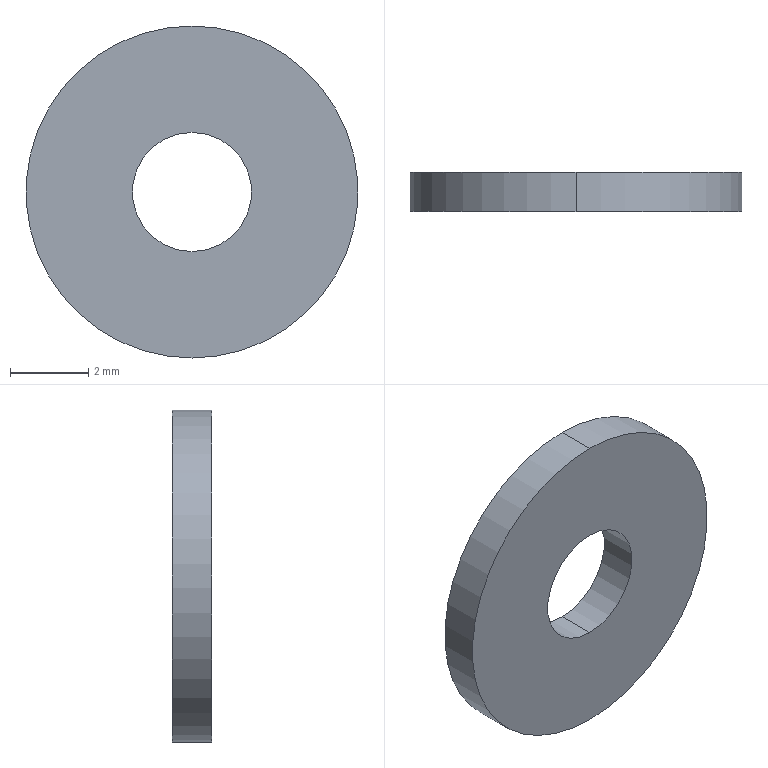Part | SolidWorks | features Extrusion 1 | 1 solid | 6 faces | box 8.5 x 1 x 8.5 mm | volume 49.439 mm3 | cylinder 4 | plane 2 | commonest cylinder face diameters 3.05 x2 8.5 x2
STEP:
#1=CARTESIAN_POINT('',(0.,1.,-1.525));
#2=VERTEX_POINT('',#1);
#3=CARTESIAN_POINT('',(0.,1.,1.525));
#4=VERTEX_POINT('',#3);
#5=CARTESIAN_POINT('',(0.,1.,0.));
#6=DIRECTION('',(0.,1.,0.));
#7=DIRECTION('',(0.,0.,1.));
#8=AXIS2_PLACEMENT_3D('',#5,#6,#7);
#9=CIRCLE('',#8,1.525);
#10=EDGE_CURVE('',#2,#4,#9,.T.);
#11=ORIENTED_EDGE('',*,*,#10,.T.);
#12=CARTESIAN_POINT('',(0.,0.,1.525));
#13=VERTEX_POINT('',#12);
#14=CARTESIAN_POINT('',(0.,1.,1.525));
#15=DIRECTION('',(0.,-1.,0.));
#16=VECTOR('',#15,1000.);
#17=LINE('',#14,#16);
#18=EDGE_CURVE('',#4,#13,#17,.T.);
#19=ORIENTED_EDGE('',*,*,#18,.T.);
#20=CARTESIAN_POINT('',(0.,0.,-1.525));
#21=VERTEX_POINT('',#20);
#22=CARTESIAN_POINT('',(0.,0.,0.));
#23=DIRECTION('',(0.,1.,0.));
#24=DIRECTION('',(0.,0.,1.));
#25=AXIS2_PLACEMENT_3D('',#22,#23,#24);
#26=CIRCLE('',#25,1.525);
#27=EDGE_CURVE('',#21,#13,#26,.T.);
#28=ORIENTED_EDGE('',*,*,#27,.F.);
#29=CARTESIAN_POINT('',(0.,1.,-1.525));
#30=DIRECTION('',(0.,-1.,0.));
#31=VECTOR('',#30,1000.);
#32=LINE('',#29,#31);
#33=EDGE_CURVE('',#2,#21,#32,.T.);
#34=ORIENTED_EDGE('',*,*,#33,.F.);
#35=EDGE_LOOP('',(#11,#19,#28,#34));
#36=FACE_OUTER_BOUND('',#35,.T.);
#37=CARTESIAN_POINT('',(0.,1.,0.));
#38=DIRECTION('',(0.,-1.,0.));
#39=DIRECTION('',(0.,0.,-1.));
#40=AXIS2_PLACEMENT_3D('',#37,#38,#39);
#41=CYLINDRICAL_SURFACE('',#40,1.525);
#42=ADVANCED_FACE('',(#36),#41,.F.);
#43=CARTESIAN_POINT('',(0.,1.,4.25));
#44=VERTEX_POINT('',#43);
#45=CARTESIAN_POINT('',(0.,1.,-4.25));
#46=VERTEX_POINT('',#45);
#47=CARTESIAN_POINT('',(0.,1.,0.));
#48=DIRECTION('',(0.,1.,0.));
#49=DIRECTION('',(0.,0.,1.));
#50=AXIS2_PLACEMENT_3D('',#47,#48,#49);
#51=CIRCLE('',#50,4.25);
#52=EDGE_CURVE('',#44,#46,#51,.T.);
#53=ORIENTED_EDGE('',*,*,#52,.F.);
#54=CARTESIAN_POINT('',(0.,0.,4.25));
#55=VERTEX_POINT('',#54);
#56=CARTESIAN_POINT('',(0.,1.,4.25));
#57=DIRECTION('',(0.,-1.,0.));
#58=VECTOR('',#57,1000.);
#59=LINE('',#56,#58);
#60=EDGE_CURVE('',#44,#55,#59,.T.);
#61=ORIENTED_EDGE('',*,*,#60,.T.);
#62=CARTESIAN_POINT('',(0.,0.,-4.25));
#63=VERTEX_POINT('',#62);
#64=CARTESIAN_POINT('',(0.,0.,0.));
#65=DIRECTION('',(0.,1.,0.));
#66=DIRECTION('',(0.,0.,1.));
#67=AXIS2_PLACEMENT_3D('',#64,#65,#66);
#68=CIRCLE('',#67,4.25);
#69=EDGE_CURVE('',#55,#63,#68,.T.);
#70=ORIENTED_EDGE('',*,*,#69,.T.);
#71=CARTESIAN_POINT('',(0.,1.,-4.25));
#72=DIRECTION('',(0.,-1.,0.));
#73=VECTOR('',#72,1000.);
#74=LINE('',#71,#73);
#75=EDGE_CURVE('',#46,#63,#74,.T.);
#76=ORIENTED_EDGE('',*,*,#75,.F.);
#77=EDGE_LOOP('',(#53,#61,#70,#76));
#78=FACE_OUTER_BOUND('',#77,.T.);
#79=CARTESIAN_POINT('',(0.,1.,0.));
#80=DIRECTION('',(0.,-1.,0.));
#81=DIRECTION('',(0.,0.,-1.));
#82=AXIS2_PLACEMENT_3D('',#79,#80,#81);
#83=CYLINDRICAL_SURFACE('',#82,4.25);
#84=ADVANCED_FACE('',(#78),#83,.T.);
#85=CARTESIAN_POINT('',(0.,1.,0.));
#86=DIRECTION('',(0.,1.,0.));
#87=DIRECTION('',(0.,0.,1.));
#88=AXIS2_PLACEMENT_3D('',#85,#86,#87);
#89=CIRCLE('',#88,4.25);
#90=EDGE_CURVE('',#46,#44,#89,.T.);
#91=ORIENTED_EDGE('',*,*,#90,.T.);
#92=ORIENTED_EDGE('',*,*,#52,.T.);
#93=EDGE_LOOP('',(#91,#92));
#94=FACE_OUTER_BOUND('',#93,.T.);
#95=ORIENTED_EDGE('',*,*,#10,.F.);
#96=CARTESIAN_POINT('',(0.,1.,0.));
#97=DIRECTION('',(0.,1.,0.));
#98=DIRECTION('',(0.,0.,1.));
#99=AXIS2_PLACEMENT_3D('',#96,#97,#98);
#100=CIRCLE('',#99,1.525);
#101=EDGE_CURVE('',#4,#2,#100,.T.);
#102=ORIENTED_EDGE('',*,*,#101,.F.);
#103=EDGE_LOOP('',(#95,#102));
#104=FACE_BOUND('',#103,.T.);
#105=CARTESIAN_POINT('',(0.,1.,0.));
#106=DIRECTION('',(0.,1.,0.));
#107=DIRECTION('',(0.,0.,1.));
#108=AXIS2_PLACEMENT_3D('',#105,#106,#107);
#109=PLANE('',#108);
#110=ADVANCED_FACE('',(#94,#104),#109,.T.);
#111=CARTESIAN_POINT('',(0.,0.,0.));
#112=DIRECTION('',(0.,1.,0.));
#113=DIRECTION('',(0.,0.,1.));
#114=AXIS2_PLACEMENT_3D('',#111,#112,#113);
#115=CIRCLE('',#114,4.25);
#116=EDGE_CURVE('',#63,#55,#115,.T.);
#117=ORIENTED_EDGE('',*,*,#116,.F.);
#118=ORIENTED_EDGE('',*,*,#69,.F.);
#119=EDGE_LOOP('',(#117,#118));
#120=FACE_OUTER_BOUND('',#119,.T.);
#121=ORIENTED_EDGE('',*,*,#27,.T.);
#122=CARTESIAN_POINT('',(0.,0.,0.));
#123=DIRECTION('',(0.,1.,0.));
#124=DIRECTION('',(0.,0.,1.));
#125=AXIS2_PLACEMENT_3D('',#122,#123,#124);
#126=CIRCLE('',#125,1.525);
#127=EDGE_CURVE('',#13,#21,#126,.T.);
#128=ORIENTED_EDGE('',*,*,#127,.T.);
#129=EDGE_LOOP('',(#121,#128));
#130=FACE_BOUND('',#129,.T.);
#131=CARTESIAN_POINT('',(0.,0.,0.));
#132=DIRECTION('',(0.,1.,0.));
#133=DIRECTION('',(0.,0.,1.));
#134=AXIS2_PLACEMENT_3D('',#131,#132,#133);
#135=PLANE('',#134);
#136=ADVANCED_FACE('',(#120,#130),#135,.F.);
#137=ORIENTED_EDGE('',*,*,#60,.F.);
#138=ORIENTED_EDGE('',*,*,#90,.F.);
#139=ORIENTED_EDGE('',*,*,#75,.T.);
#140=ORIENTED_EDGE('',*,*,#116,.T.);
#141=EDGE_LOOP('',(#137,#138,#139,#140));
#142=FACE_OUTER_BOUND('',#141,.T.);
#143=CARTESIAN_POINT('',(0.,1.,0.));
#144=DIRECTION('',(0.,-1.,0.));
#145=DIRECTION('',(0.,0.,-1.));
#146=AXIS2_PLACEMENT_3D('',#143,#144,#145);
#147=CYLINDRICAL_SURFACE('',#146,4.25);
#148=ADVANCED_FACE('',(#142),#147,.T.);
#149=ORIENTED_EDGE('',*,*,#18,.F.);
#150=ORIENTED_EDGE('',*,*,#101,.T.);
#151=ORIENTED_EDGE('',*,*,#33,.T.);
#152=ORIENTED_EDGE('',*,*,#127,.F.);
#153=EDGE_LOOP('',(#149,#150,#151,#152));
#154=FACE_OUTER_BOUND('',#153,.T.);
#155=CARTESIAN_POINT('',(0.,1.,0.));
#156=DIRECTION('',(0.,-1.,0.));
#157=DIRECTION('',(0.,0.,-1.));
#158=AXIS2_PLACEMENT_3D('',#155,#156,#157);
#159=CYLINDRICAL_SURFACE('',#158,1.525);
#160=ADVANCED_FACE('',(#154),#159,.F.);
#161=CLOSED_SHELL('',(#42,#84,#110,#136,#148,#160));
#162=MANIFOLD_SOLID_BREP('',#161);
#163=CARTESIAN_POINT('',(0.,0.,0.));
#164=DIRECTION('',(0.,0.,1.));
#165=DIRECTION('',(1.,0.,0.));
#166=AXIS2_PLACEMENT_3D('',#163,#164,#165);
#167=(LENGTH_UNIT()NAMED_UNIT(*)SI_UNIT(.MILLI.,.METRE.));
#168=UNCERTAINTY_MEASURE_WITH_UNIT(LENGTH_MEASURE(0.00001),#167,'','');
#169=(NAMED_UNIT(*)PLANE_ANGLE_UNIT()SI_UNIT($,.RADIAN.));
#170=(NAMED_UNIT(*)SI_UNIT($,.STERADIAN.)SOLID_ANGLE_UNIT());
#171=(GEOMETRIC_REPRESENTATION_CONTEXT(3)GLOBAL_UNCERTAINTY_ASSIGNED_CONTEXT((#168))GLOBAL_UNIT_ASSIGNED_CONTEXT((#167,#169,#170))REPRESENTATION_CONTEXT('',''));
#172=ADVANCED_BREP_SHAPE_REPRESENTATION('',(#162,#166),#171);